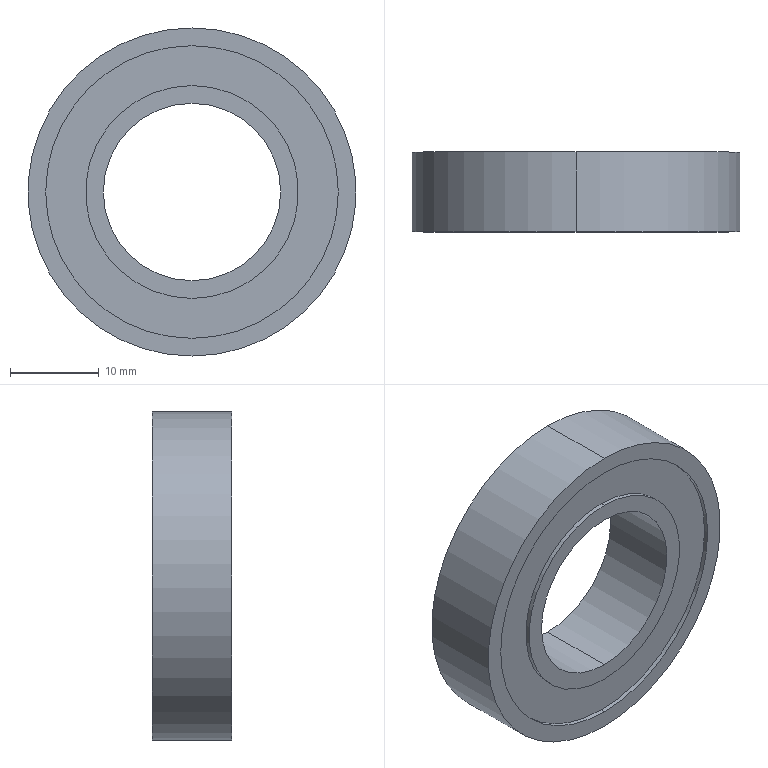Part | STEP file | Bearing 6904 | 1 solid | 18 faces | box 37 x 9 x 37 mm | volume 6447 mm3 | cylinder 12 | plane 6 | commonest cylinder face diameters 24 x4 33 x4 20 x2 37 x2
STEP:
#1=CARTESIAN_POINT('',(0.,0.,0.));
#2=DIRECTION('',(0.,0.,1.));
#3=DIRECTION('',(1.,0.,0.));
#4=AXIS2_PLACEMENT_3D('',#1,#2,#3);
#5=CARTESIAN_POINT('',(0.,-4.,12.));
#6=VERTEX_POINT('',#5);
#7=CARTESIAN_POINT('',(0.,-4.,-12.));
#8=VERTEX_POINT('',#7);
#9=CARTESIAN_POINT('',(0.,-4.,0.));
#10=DIRECTION('',(0.,1.,0.));
#11=DIRECTION('',(0.,0.,1.));
#12=AXIS2_PLACEMENT_3D('',#9,#10,#11);
#13=CIRCLE('',#12,12.);
#14=CARTESIAN_POINT('',(0.,-4.,0.));
#15=DIRECTION('',(0.,-1.,0.));
#16=DIRECTION('',(0.,0.,-1.));
#17=AXIS2_PLACEMENT_3D('',#14,#15,#16);
#18=CYLINDRICAL_SURFACE('',#17,12.);
#19=CARTESIAN_POINT('',(3.142,0.));
#20=DIRECTION('',(-1.,0.));
#21=VECTOR('',#20,1.);
#22=LINE('',#19,#21);
#23=(GEOMETRIC_REPRESENTATION_CONTEXT(2)PARAMETRIC_REPRESENTATION_CONTEXT()REPRESENTATION_CONTEXT('',''));
#24=DEFINITIONAL_REPRESENTATION('',(#22),#23);
#25=PCURVE('',#18,#24);
#26=CARTESIAN_POINT('',(0.,-4.,0.));
#27=DIRECTION('',(0.,-1.,0.));
#28=DIRECTION('',(0.,0.,1.));
#29=AXIS2_PLACEMENT_3D('',#26,#27,#28);
#30=PLANE('',#29);
#31=CARTESIAN_POINT('',(12.,0.));
#32=CARTESIAN_POINT('',(12.,-20.785));
#33=CARTESIAN_POINT('',(-6.,-10.392));
#34=CARTESIAN_POINT('',(-24.,0.));
#35=CARTESIAN_POINT('',(-6.,10.392));
#36=CARTESIAN_POINT('',(12.,20.785));
#37=CARTESIAN_POINT('',(12.,0.));
#38=(BOUNDED_CURVE()B_SPLINE_CURVE(2,(#31,#32,#33,#34,#35,#36,#37),.UNSPECIFIED.,.T.,.F.)B_SPLINE_CURVE_WITH_KNOTS((1,2,2,2,2,1),(-2.094,0.,2.094,4.189,6.283,8.378),.UNSPECIFIED.)CURVE()GEOMETRIC_REPRESENTATION_ITEM()RATIONAL_B_SPLINE_CURVE((1.,0.5,1.,0.5,1.,0.5,1.))REPRESENTATION_ITEM(''));
#39=(GEOMETRIC_REPRESENTATION_CONTEXT(2)PARAMETRIC_REPRESENTATION_CONTEXT()REPRESENTATION_CONTEXT('',''));
#40=DEFINITIONAL_REPRESENTATION('',(#38),#39);
#41=PCURVE('',#30,#40);
#42=SURFACE_CURVE('',#13,(#25,#41),.PCURVE_S1.);
#43=EDGE_CURVE('',#6,#8,#42,.T.);
#44=ORIENTED_EDGE('',*,*,#43,.F.);
#45=CARTESIAN_POINT('',(0.,-4.5,12.));
#46=VERTEX_POINT('',#45);
#47=CARTESIAN_POINT('',(0.,-4.,12.));
#48=DIRECTION('',(0.,-1.,0.));
#49=VECTOR('',#48,1.);
#50=LINE('',#47,#49);
#51=CARTESIAN_POINT('',(3.142,0.));
#52=DIRECTION('',(0.,1.));
#53=VECTOR('',#52,1.);
#54=LINE('',#51,#53);
#55=(GEOMETRIC_REPRESENTATION_CONTEXT(2)PARAMETRIC_REPRESENTATION_CONTEXT()REPRESENTATION_CONTEXT('',''));
#56=DEFINITIONAL_REPRESENTATION('',(#54),#55);
#57=PCURVE('',#18,#56);
#58=CARTESIAN_POINT('',(0.,-4.,0.));
#59=DIRECTION('',(0.,-1.,0.));
#60=DIRECTION('',(0.,0.,-1.));
#61=AXIS2_PLACEMENT_3D('',#58,#59,#60);
#62=CYLINDRICAL_SURFACE('',#61,12.);
#63=CARTESIAN_POINT('',(3.142,0.));
#64=DIRECTION('',(0.,1.));
#65=VECTOR('',#64,1.);
#66=LINE('',#63,#65);
#67=(GEOMETRIC_REPRESENTATION_CONTEXT(2)PARAMETRIC_REPRESENTATION_CONTEXT()REPRESENTATION_CONTEXT('',''));
#68=DEFINITIONAL_REPRESENTATION('',(#66),#67);
#69=PCURVE('',#62,#68);
#70=SURFACE_CURVE('',#50,(#57,#69),.PCURVE_S1.);
#71=EDGE_CURVE('',#6,#46,#70,.T.);
#72=ORIENTED_EDGE('',*,*,#71,.T.);
#73=CARTESIAN_POINT('',(0.,-4.5,-12.));
#74=VERTEX_POINT('',#73);
#75=CARTESIAN_POINT('',(0.,-4.5,0.));
#76=DIRECTION('',(0.,1.,0.));
#77=DIRECTION('',(0.,0.,1.));
#78=AXIS2_PLACEMENT_3D('',#75,#76,#77);
#79=CIRCLE('',#78,12.);
#80=CARTESIAN_POINT('',(3.142,0.5));
#81=DIRECTION('',(-1.,0.));
#82=VECTOR('',#81,1.);
#83=LINE('',#80,#82);
#84=(GEOMETRIC_REPRESENTATION_CONTEXT(2)PARAMETRIC_REPRESENTATION_CONTEXT()REPRESENTATION_CONTEXT('',''));
#85=DEFINITIONAL_REPRESENTATION('',(#83),#84);
#86=PCURVE('',#18,#85);
#87=CARTESIAN_POINT('',(0.,-4.5,0.));
#88=DIRECTION('',(0.,1.,0.));
#89=DIRECTION('',(0.,0.,1.));
#90=AXIS2_PLACEMENT_3D('',#87,#88,#89);
#91=PLANE('',#90);
#92=CARTESIAN_POINT('',(0.,0.));
#93=DIRECTION('',(1.,0.));
#94=AXIS2_PLACEMENT_2D('',#92,#93);
#95=CIRCLE('',#94,12.);
#96=(GEOMETRIC_REPRESENTATION_CONTEXT(2)PARAMETRIC_REPRESENTATION_CONTEXT()REPRESENTATION_CONTEXT('',''));
#97=DEFINITIONAL_REPRESENTATION('',(#95),#96);
#98=PCURVE('',#91,#97);
#99=SURFACE_CURVE('',#79,(#86,#98),.PCURVE_S1.);
#100=EDGE_CURVE('',#46,#74,#99,.T.);
#101=ORIENTED_EDGE('',*,*,#100,.T.);
#102=CARTESIAN_POINT('',(0.,-4.,-12.));
#103=DIRECTION('',(0.,-1.,0.));
#104=VECTOR('',#103,1.);
#105=LINE('',#102,#104);
#106=CARTESIAN_POINT('',(0.,0.));
#107=DIRECTION('',(0.,1.));
#108=VECTOR('',#107,1.);
#109=LINE('',#106,#108);
#110=(GEOMETRIC_REPRESENTATION_CONTEXT(2)PARAMETRIC_REPRESENTATION_CONTEXT()REPRESENTATION_CONTEXT('',''));
#111=DEFINITIONAL_REPRESENTATION('',(#109),#110);
#112=PCURVE('',#18,#111);
#113=CARTESIAN_POINT('',(6.283,0.));
#114=DIRECTION('',(0.,1.));
#115=VECTOR('',#114,1.);
#116=LINE('',#113,#115);
#117=(GEOMETRIC_REPRESENTATION_CONTEXT(2)PARAMETRIC_REPRESENTATION_CONTEXT()REPRESENTATION_CONTEXT('',''));
#118=DEFINITIONAL_REPRESENTATION('',(#116),#117);
#119=PCURVE('',#62,#118);
#120=SURFACE_CURVE('',#105,(#112,#119),.PCURVE_S1.);
#121=EDGE_CURVE('',#8,#74,#120,.T.);
#122=ORIENTED_EDGE('',*,*,#121,.F.);
#123=EDGE_LOOP('',(#44,#72,#101,#122));
#124=FACE_BOUND('',#123,.T.);
#125=ADVANCED_FACE('',(#124),#18,.T.);
#126=CARTESIAN_POINT('',(0.,-4.,-16.5));
#127=VERTEX_POINT('',#126);
#128=CARTESIAN_POINT('',(0.,-4.5,-16.5));
#129=VERTEX_POINT('',#128);
#130=CARTESIAN_POINT('',(0.,-4.,-16.5));
#131=DIRECTION('',(0.,-1.,0.));
#132=VECTOR('',#131,1.);
#133=LINE('',#130,#132);
#134=CARTESIAN_POINT('',(0.,-4.,0.));
#135=DIRECTION('',(0.,-1.,0.));
#136=DIRECTION('',(0.,0.,-1.));
#137=AXIS2_PLACEMENT_3D('',#134,#135,#136);
#138=CYLINDRICAL_SURFACE('',#137,16.5);
#139=CARTESIAN_POINT('',(6.283,0.));
#140=DIRECTION('',(0.,1.));
#141=VECTOR('',#140,1.);
#142=LINE('',#139,#141);
#143=(GEOMETRIC_REPRESENTATION_CONTEXT(2)PARAMETRIC_REPRESENTATION_CONTEXT()REPRESENTATION_CONTEXT('',''));
#144=DEFINITIONAL_REPRESENTATION('',(#142),#143);
#145=PCURVE('',#138,#144);
#146=CARTESIAN_POINT('',(0.,-4.,0.));
#147=DIRECTION('',(0.,-1.,0.));
#148=DIRECTION('',(0.,0.,-1.));
#149=AXIS2_PLACEMENT_3D('',#146,#147,#148);
#150=CYLINDRICAL_SURFACE('',#149,16.5);
#151=CARTESIAN_POINT('',(0.,0.));
#152=DIRECTION('',(0.,1.));
#153=VECTOR('',#152,1.);
#154=LINE('',#151,#153);
#155=(GEOMETRIC_REPRESENTATION_CONTEXT(2)PARAMETRIC_REPRESENTATION_CONTEXT()REPRESENTATION_CONTEXT('',''));
#156=DEFINITIONAL_REPRESENTATION('',(#154),#155);
#157=PCURVE('',#150,#156);
#158=SURFACE_CURVE('',#133,(#145,#157),.PCURVE_S1.);
#159=EDGE_CURVE('',#127,#129,#158,.T.);
#160=ORIENTED_EDGE('',*,*,#159,.T.);
#161=CARTESIAN_POINT('',(0.,-4.5,16.5));
#162=VERTEX_POINT('',#161);
#163=CARTESIAN_POINT('',(0.,-4.5,0.));
#164=DIRECTION('',(0.,1.,0.));
#165=DIRECTION('',(0.,0.,1.));
#166=AXIS2_PLACEMENT_3D('',#163,#164,#165);
#167=CIRCLE('',#166,16.5);
#168=CARTESIAN_POINT('',(9.425,0.5));
#169=DIRECTION('',(-1.,0.));
#170=VECTOR('',#169,1.);
#171=LINE('',#168,#170);
#172=(GEOMETRIC_REPRESENTATION_CONTEXT(2)PARAMETRIC_REPRESENTATION_CONTEXT()REPRESENTATION_CONTEXT('',''));
#173=DEFINITIONAL_REPRESENTATION('',(#171),#172);
#174=PCURVE('',#138,#173);
#175=CARTESIAN_POINT('',(0.,-4.5,0.));
#176=DIRECTION('',(0.,1.,0.));
#177=DIRECTION('',(0.,0.,1.));
#178=AXIS2_PLACEMENT_3D('',#175,#176,#177);
#179=PLANE('',#178);
#180=CARTESIAN_POINT('',(0.,0.));
#181=DIRECTION('',(1.,0.));
#182=AXIS2_PLACEMENT_2D('',#180,#181);
#183=CIRCLE('',#182,16.5);
#184=(GEOMETRIC_REPRESENTATION_CONTEXT(2)PARAMETRIC_REPRESENTATION_CONTEXT()REPRESENTATION_CONTEXT('',''));
#185=DEFINITIONAL_REPRESENTATION('',(#183),#184);
#186=PCURVE('',#179,#185);
#187=SURFACE_CURVE('',#167,(#174,#186),.PCURVE_S1.);
#188=EDGE_CURVE('',#129,#162,#187,.T.);
#189=ORIENTED_EDGE('',*,*,#188,.T.);
#190=CARTESIAN_POINT('',(0.,-4.,16.5));
#191=VERTEX_POINT('',#190);
#192=CARTESIAN_POINT('',(0.,-4.,16.5));
#193=DIRECTION('',(0.,-1.,0.));
#194=VECTOR('',#193,1.);
#195=LINE('',#192,#194);
#196=CARTESIAN_POINT('',(3.142,0.));
#197=DIRECTION('',(0.,1.));
#198=VECTOR('',#197,1.);
#199=LINE('',#196,#198);
#200=(GEOMETRIC_REPRESENTATION_CONTEXT(2)PARAMETRIC_REPRESENTATION_CONTEXT()REPRESENTATION_CONTEXT('',''));
#201=DEFINITIONAL_REPRESENTATION('',(#199),#200);
#202=PCURVE('',#138,#201);
#203=CARTESIAN_POINT('',(3.142,0.));
#204=DIRECTION('',(0.,1.));
#205=VECTOR('',#204,1.);
#206=LINE('',#203,#205);
#207=(GEOMETRIC_REPRESENTATION_CONTEXT(2)PARAMETRIC_REPRESENTATION_CONTEXT()REPRESENTATION_CONTEXT('',''));
#208=DEFINITIONAL_REPRESENTATION('',(#206),#207);
#209=PCURVE('',#150,#208);
#210=SURFACE_CURVE('',#195,(#202,#209),.PCURVE_S1.);
#211=EDGE_CURVE('',#191,#162,#210,.T.);
#212=ORIENTED_EDGE('',*,*,#211,.F.);
#213=CARTESIAN_POINT('',(0.,-4.,0.));
#214=DIRECTION('',(0.,1.,0.));
#215=DIRECTION('',(0.,0.,1.));
#216=AXIS2_PLACEMENT_3D('',#213,#214,#215);
#217=CIRCLE('',#216,16.5);
#218=CARTESIAN_POINT('',(9.425,0.));
#219=DIRECTION('',(-1.,0.));
#220=VECTOR('',#219,1.);
#221=LINE('',#218,#220);
#222=(GEOMETRIC_REPRESENTATION_CONTEXT(2)PARAMETRIC_REPRESENTATION_CONTEXT()REPRESENTATION_CONTEXT('',''));
#223=DEFINITIONAL_REPRESENTATION('',(#221),#222);
#224=PCURVE('',#138,#223);
#225=CARTESIAN_POINT('',(16.5,0.));
#226=CARTESIAN_POINT('',(16.5,-28.579));
#227=CARTESIAN_POINT('',(-8.25,-14.289));
#228=CARTESIAN_POINT('',(-33.,0.));
#229=CARTESIAN_POINT('',(-8.25,14.289));
#230=CARTESIAN_POINT('',(16.5,28.579));
#231=CARTESIAN_POINT('',(16.5,0.));
#232=(BOUNDED_CURVE()B_SPLINE_CURVE(2,(#225,#226,#227,#228,#229,#230,#231),.UNSPECIFIED.,.T.,.F.)B_SPLINE_CURVE_WITH_KNOTS((1,2,2,2,2,1),(-2.094,0.,2.094,4.189,6.283,8.378),.UNSPECIFIED.)CURVE()GEOMETRIC_REPRESENTATION_ITEM()RATIONAL_B_SPLINE_CURVE((1.,0.5,1.,0.5,1.,0.5,1.))REPRESENTATION_ITEM(''));
#233=(GEOMETRIC_REPRESENTATION_CONTEXT(2)PARAMETRIC_REPRESENTATION_CONTEXT()REPRESENTATION_CONTEXT('',''));
#234=DEFINITIONAL_REPRESENTATION('',(#232),#233);
#235=PCURVE('',#30,#234);
#236=SURFACE_CURVE('',#217,(#224,#235),.PCURVE_S1.);
#237=EDGE_CURVE('',#127,#191,#236,.T.);
#238=ORIENTED_EDGE('',*,*,#237,.F.);
#239=EDGE_LOOP('',(#160,#189,#212,#238));
#240=FACE_BOUND('',#239,.F.);
#241=ADVANCED_FACE('',(#240),#138,.F.);
#242=CARTESIAN_POINT('',(0.,4.,12.));
#243=VERTEX_POINT('',#242);
#244=CARTESIAN_POINT('',(0.,4.,-12.));
#245=VERTEX_POINT('',#244);
#246=CARTESIAN_POINT('',(0.,4.,0.));
#247=DIRECTION('',(0.,1.,0.));
#248=DIRECTION('',(0.,0.,1.));
#249=AXIS2_PLACEMENT_3D('',#246,#247,#248);
#250=CIRCLE('',#249,12.);
#251=CARTESIAN_POINT('',(0.,4.,0.));
#252=DIRECTION('',(0.,1.,0.));
#253=DIRECTION('',(0.,0.,1.));
#254=AXIS2_PLACEMENT_3D('',#251,#252,#253);
#255=CYLINDRICAL_SURFACE('',#254,12.);
#256=CARTESIAN_POINT('',(0.,0.));
#257=DIRECTION('',(1.,0.));
#258=VECTOR('',#257,1.);
#259=LINE('',#256,#258);
#260=(GEOMETRIC_REPRESENTATION_CONTEXT(2)PARAMETRIC_REPRESENTATION_CONTEXT()REPRESENTATION_CONTEXT('',''));
#261=DEFINITIONAL_REPRESENTATION('',(#259),#260);
#262=PCURVE('',#255,#261);
#263=CARTESIAN_POINT('',(0.,4.,0.));
#264=DIRECTION('',(0.,1.,0.));
#265=DIRECTION('',(0.,0.,1.));
#266=AXIS2_PLACEMENT_3D('',#263,#264,#265);
#267=PLANE('',#266);
#268=CARTESIAN_POINT('',(0.,0.));
#269=DIRECTION('',(1.,0.));
#270=AXIS2_PLACEMENT_2D('',#268,#269);
#271=CIRCLE('',#270,12.);
#272=(GEOMETRIC_REPRESENTATION_CONTEXT(2)PARAMETRIC_REPRESENTATION_CONTEXT()REPRESENTATION_CONTEXT('',''));
#273=DEFINITIONAL_REPRESENTATION('',(#271),#272);
#274=PCURVE('',#267,#273);
#275=SURFACE_CURVE('',#250,(#262,#274),.PCURVE_S1.);
#276=EDGE_CURVE('',#243,#245,#275,.T.);
#277=ORIENTED_EDGE('',*,*,#276,.T.);
#278=CARTESIAN_POINT('',(0.,4.5,-12.));
#279=VERTEX_POINT('',#278);
#280=CARTESIAN_POINT('',(0.,4.,-12.));
#281=DIRECTION('',(0.,1.,0.));
#282=VECTOR('',#281,1.);
#283=LINE('',#280,#282);
#284=CARTESIAN_POINT('',(3.142,0.));
#285=DIRECTION('',(0.,1.));
#286=VECTOR('',#285,1.);
#287=LINE('',#284,#286);
#288=(GEOMETRIC_REPRESENTATION_CONTEXT(2)PARAMETRIC_REPRESENTATION_CONTEXT()REPRESENTATION_CONTEXT('',''));
#289=DEFINITIONAL_REPRESENTATION('',(#287),#288);
#290=PCURVE('',#255,#289);
#291=CARTESIAN_POINT('',(0.,4.,0.));
#292=DIRECTION('',(0.,1.,0.));
#293=DIRECTION('',(0.,0.,1.));
#294=AXIS2_PLACEMENT_3D('',#291,#292,#293);
#295=CYLINDRICAL_SURFACE('',#294,12.);
#296=CARTESIAN_POINT('',(3.142,0.));
#297=DIRECTION('',(0.,1.));
#298=VECTOR('',#297,1.);
#299=LINE('',#296,#298);
#300=(GEOMETRIC_REPRESENTATION_CONTEXT(2)PARAMETRIC_REPRESENTATION_CONTEXT()REPRESENTATION_CONTEXT('',''));
#301=DEFINITIONAL_REPRESENTATION('',(#299),#300);
#302=PCURVE('',#295,#301);
#303=SURFACE_CURVE('',#283,(#290,#302),.PCURVE_S1.);
#304=EDGE_CURVE('',#245,#279,#303,.T.);
#305=ORIENTED_EDGE('',*,*,#304,.T.);
#306=CARTESIAN_POINT('',(0.,4.5,12.));
#307=VERTEX_POINT('',#306);
#308=CARTESIAN_POINT('',(0.,4.5,0.));
#309=DIRECTION('',(0.,1.,0.));
#310=DIRECTION('',(0.,0.,1.));
#311=AXIS2_PLACEMENT_3D('',#308,#309,#310);
#312=CIRCLE('',#311,12.);
#313=CARTESIAN_POINT('',(0.,0.5));
#314=DIRECTION('',(1.,0.));
#315=VECTOR('',#314,1.);
#316=LINE('',#313,#315);
#317=(GEOMETRIC_REPRESENTATION_CONTEXT(2)PARAMETRIC_REPRESENTATION_CONTEXT()REPRESENTATION_CONTEXT('',''));
#318=DEFINITIONAL_REPRESENTATION('',(#316),#317);
#319=PCURVE('',#255,#318);
#320=CARTESIAN_POINT('',(0.,4.5,0.));
#321=DIRECTION('',(0.,1.,0.));
#322=DIRECTION('',(0.,0.,1.));
#323=AXIS2_PLACEMENT_3D('',#320,#321,#322);
#324=PLANE('',#323);
#325=CARTESIAN_POINT('',(0.,0.));
#326=DIRECTION('',(1.,0.));
#327=AXIS2_PLACEMENT_2D('',#325,#326);
#328=CIRCLE('',#327,12.);
#329=(GEOMETRIC_REPRESENTATION_CONTEXT(2)PARAMETRIC_REPRESENTATION_CONTEXT()REPRESENTATION_CONTEXT('',''));
#330=DEFINITIONAL_REPRESENTATION('',(#328),#329);
#331=PCURVE('',#324,#330);
#332=SURFACE_CURVE('',#312,(#319,#331),.PCURVE_S1.);
#333=EDGE_CURVE('',#307,#279,#332,.T.);
#334=ORIENTED_EDGE('',*,*,#333,.F.);
#335=CARTESIAN_POINT('',(0.,4.,12.));
#336=DIRECTION('',(0.,1.,0.));
#337=VECTOR('',#336,1.);
#338=LINE('',#335,#337);
#339=CARTESIAN_POINT('',(0.,0.));
#340=DIRECTION('',(0.,1.));
#341=VECTOR('',#340,1.);
#342=LINE('',#339,#341);
#343=(GEOMETRIC_REPRESENTATION_CONTEXT(2)PARAMETRIC_REPRESENTATION_CONTEXT()REPRESENTATION_CONTEXT('',''));
#344=DEFINITIONAL_REPRESENTATION('',(#342),#343);
#345=PCURVE('',#255,#344);
#346=CARTESIAN_POINT('',(6.283,0.));
#347=DIRECTION('',(0.,1.));
#348=VECTOR('',#347,1.);
#349=LINE('',#346,#348);
#350=(GEOMETRIC_REPRESENTATION_CONTEXT(2)PARAMETRIC_REPRESENTATION_CONTEXT()REPRESENTATION_CONTEXT('',''));
#351=DEFINITIONAL_REPRESENTATION('',(#349),#350);
#352=PCURVE('',#295,#351);
#353=SURFACE_CURVE('',#338,(#345,#352),.PCURVE_S1.);
#354=EDGE_CURVE('',#243,#307,#353,.T.);
#355=ORIENTED_EDGE('',*,*,#354,.F.);
#356=EDGE_LOOP('',(#277,#305,#334,#355));
#357=FACE_BOUND('',#356,.T.);
#358=ADVANCED_FACE('',(#357),#255,.T.);
#359=CARTESIAN_POINT('',(0.,4.,16.5));
#360=VERTEX_POINT('',#359);
#361=CARTESIAN_POINT('',(0.,4.5,16.5));
#362=VERTEX_POINT('',#361);
#363=CARTESIAN_POINT('',(0.,4.,16.5));
#364=DIRECTION('',(0.,1.,0.));
#365=VECTOR('',#364,1.);
#366=LINE('',#363,#365);
#367=CARTESIAN_POINT('',(0.,4.,0.));
#368=DIRECTION('',(0.,1.,0.));
#369=DIRECTION('',(0.,0.,1.));
#370=AXIS2_PLACEMENT_3D('',#367,#368,#369);
#371=CYLINDRICAL_SURFACE('',#370,16.5);
#372=CARTESIAN_POINT('',(6.283,0.));
#373=DIRECTION('',(0.,1.));
#374=VECTOR('',#373,1.);
#375=LINE('',#372,#374);
#376=(GEOMETRIC_REPRESENTATION_CONTEXT(2)PARAMETRIC_REPRESENTATION_CONTEXT()REPRESENTATION_CONTEXT('',''));
#377=DEFINITIONAL_REPRESENTATION('',(#375),#376);
#378=PCURVE('',#371,#377);
#379=CARTESIAN_POINT('',(0.,4.,0.));
#380=DIRECTION('',(0.,1.,0.));
#381=DIRECTION('',(0.,0.,1.));
#382=AXIS2_PLACEMENT_3D('',#379,#380,#381);
#383=CYLINDRICAL_SURFACE('',#382,16.5);
#384=CARTESIAN_POINT('',(0.,0.));
#385=DIRECTION('',(0.,1.));
#386=VECTOR('',#385,1.);
#387=LINE('',#384,#386);
#388=(GEOMETRIC_REPRESENTATION_CONTEXT(2)PARAMETRIC_REPRESENTATION_CONTEXT()REPRESENTATION_CONTEXT('',''));
#389=DEFINITIONAL_REPRESENTATION('',(#387),#388);
#390=PCURVE('',#383,#389);
#391=SURFACE_CURVE('',#366,(#378,#390),.PCURVE_S1.);
#392=EDGE_CURVE('',#360,#362,#391,.T.);
#393=ORIENTED_EDGE('',*,*,#392,.T.);
#394=CARTESIAN_POINT('',(0.,4.5,-16.5));
#395=VERTEX_POINT('',#394);
#396=CARTESIAN_POINT('',(0.,4.5,0.));
#397=DIRECTION('',(0.,1.,0.));
#398=DIRECTION('',(0.,0.,1.));
#399=AXIS2_PLACEMENT_3D('',#396,#397,#398);
#400=CIRCLE('',#399,16.5);
#401=CARTESIAN_POINT('',(0.,0.5));
#402=DIRECTION('',(1.,0.));
#403=VECTOR('',#402,1.);
#404=LINE('',#401,#403);
#405=(GEOMETRIC_REPRESENTATION_CONTEXT(2)PARAMETRIC_REPRESENTATION_CONTEXT()REPRESENTATION_CONTEXT('',''));
#406=DEFINITIONAL_REPRESENTATION('',(#404),#405);
#407=PCURVE('',#371,#406);
#408=CARTESIAN_POINT('',(0.,4.5,0.));
#409=DIRECTION('',(0.,1.,0.));
#410=DIRECTION('',(0.,0.,1.));
#411=AXIS2_PLACEMENT_3D('',#408,#409,#410);
#412=PLANE('',#411);
#413=CARTESIAN_POINT('',(0.,0.));
#414=DIRECTION('',(1.,0.));
#415=AXIS2_PLACEMENT_2D('',#413,#414);
#416=CIRCLE('',#415,16.5);
#417=(GEOMETRIC_REPRESENTATION_CONTEXT(2)PARAMETRIC_REPRESENTATION_CONTEXT()REPRESENTATION_CONTEXT('',''));
#418=DEFINITIONAL_REPRESENTATION('',(#416),#417);
#419=PCURVE('',#412,#418);
#420=SURFACE_CURVE('',#400,(#407,#419),.PCURVE_S1.);
#421=EDGE_CURVE('',#395,#362,#420,.T.);
#422=ORIENTED_EDGE('',*,*,#421,.F.);
#423=CARTESIAN_POINT('',(0.,4.,-16.5));
#424=VERTEX_POINT('',#423);
#425=CARTESIAN_POINT('',(0.,4.,-16.5));
#426=DIRECTION('',(0.,1.,0.));
#427=VECTOR('',#426,1.);
#428=LINE('',#425,#427);
#429=CARTESIAN_POINT('',(3.142,0.));
#430=DIRECTION('',(0.,1.));
#431=VECTOR('',#430,1.);
#432=LINE('',#429,#431);
#433=(GEOMETRIC_REPRESENTATION_CONTEXT(2)PARAMETRIC_REPRESENTATION_CONTEXT()REPRESENTATION_CONTEXT('',''));
#434=DEFINITIONAL_REPRESENTATION('',(#432),#433);
#435=PCURVE('',#371,#434);
#436=CARTESIAN_POINT('',(3.142,0.));
#437=DIRECTION('',(0.,1.));
#438=VECTOR('',#437,1.);
#439=LINE('',#436,#438);
#440=(GEOMETRIC_REPRESENTATION_CONTEXT(2)PARAMETRIC_REPRESENTATION_CONTEXT()REPRESENTATION_CONTEXT('',''));
#441=DEFINITIONAL_REPRESENTATION('',(#439),#440);
#442=PCURVE('',#383,#441);
#443=SURFACE_CURVE('',#428,(#435,#442),.PCURVE_S1.);
#444=EDGE_CURVE('',#424,#395,#443,.T.);
#445=ORIENTED_EDGE('',*,*,#444,.F.);
#446=CARTESIAN_POINT('',(0.,4.,0.));
#447=DIRECTION('',(0.,1.,0.));
#448=DIRECTION('',(0.,0.,1.));
#449=AXIS2_PLACEMENT_3D('',#446,#447,#448);
#450=CIRCLE('',#449,16.5);
#451=CARTESIAN_POINT('',(0.,0.));
#452=DIRECTION('',(1.,0.));
#453=VECTOR('',#452,1.);
#454=LINE('',#451,#453);
#455=(GEOMETRIC_REPRESENTATION_CONTEXT(2)PARAMETRIC_REPRESENTATION_CONTEXT()REPRESENTATION_CONTEXT('',''));
#456=DEFINITIONAL_REPRESENTATION('',(#454),#455);
#457=PCURVE('',#371,#456);
#458=CARTESIAN_POINT('',(0.,0.));
#459=DIRECTION('',(1.,0.));
#460=AXIS2_PLACEMENT_2D('',#458,#459);
#461=CIRCLE('',#460,16.5);
#462=(GEOMETRIC_REPRESENTATION_CONTEXT(2)PARAMETRIC_REPRESENTATION_CONTEXT()REPRESENTATION_CONTEXT('',''));
#463=DEFINITIONAL_REPRESENTATION('',(#461),#462);
#464=PCURVE('',#267,#463);
#465=SURFACE_CURVE('',#450,(#457,#464),.PCURVE_S1.);
#466=EDGE_CURVE('',#424,#360,#465,.T.);
#467=ORIENTED_EDGE('',*,*,#466,.T.);
#468=EDGE_LOOP('',(#393,#422,#445,#467));
#469=FACE_BOUND('',#468,.F.);
#470=ADVANCED_FACE('',(#469),#371,.F.);
#471=CARTESIAN_POINT('',(0.,4.5,-10.));
#472=VERTEX_POINT('',#471);
#473=CARTESIAN_POINT('',(0.,-4.5,-10.));
#474=VERTEX_POINT('',#473);
#475=CARTESIAN_POINT('',(0.,4.5,-10.));
#476=DIRECTION('',(0.,-1.,0.));
#477=VECTOR('',#476,1.);
#478=LINE('',#475,#477);
#479=CARTESIAN_POINT('',(0.,4.5,0.));
#480=DIRECTION('',(0.,-1.,0.));
#481=DIRECTION('',(0.,0.,-1.));
#482=AXIS2_PLACEMENT_3D('',#479,#480,#481);
#483=CYLINDRICAL_SURFACE('',#482,10.);
#484=CARTESIAN_POINT('',(6.283,0.));
#485=DIRECTION('',(0.,1.));
#486=VECTOR('',#485,1.);
#487=LINE('',#484,#486);
#488=(GEOMETRIC_REPRESENTATION_CONTEXT(2)PARAMETRIC_REPRESENTATION_CONTEXT()REPRESENTATION_CONTEXT('',''));
#489=DEFINITIONAL_REPRESENTATION('',(#487),#488);
#490=PCURVE('',#483,#489);
#491=CARTESIAN_POINT('',(0.,4.5,0.));
#492=DIRECTION('',(0.,-1.,0.));
#493=DIRECTION('',(0.,0.,-1.));
#494=AXIS2_PLACEMENT_3D('',#491,#492,#493);
#495=CYLINDRICAL_SURFACE('',#494,10.);
#496=CARTESIAN_POINT('',(0.,0.));
#497=DIRECTION('',(0.,1.));
#498=VECTOR('',#497,1.);
#499=LINE('',#496,#498);
#500=(GEOMETRIC_REPRESENTATION_CONTEXT(2)PARAMETRIC_REPRESENTATION_CONTEXT()REPRESENTATION_CONTEXT('',''));
#501=DEFINITIONAL_REPRESENTATION('',(#499),#500);
#502=PCURVE('',#495,#501);
#503=SURFACE_CURVE('',#478,(#490,#502),.PCURVE_S1.);
#504=EDGE_CURVE('',#472,#474,#503,.T.);
#505=ORIENTED_EDGE('',*,*,#504,.T.);
#506=CARTESIAN_POINT('',(0.,-4.5,10.));
#507=VERTEX_POINT('',#506);
#508=CARTESIAN_POINT('',(0.,-4.5,0.));
#509=DIRECTION('',(0.,1.,0.));
#510=DIRECTION('',(0.,0.,1.));
#511=AXIS2_PLACEMENT_3D('',#508,#509,#510);
#512=CIRCLE('',#511,10.);
#513=CARTESIAN_POINT('',(9.425,9.));
#514=DIRECTION('',(-1.,0.));
#515=VECTOR('',#514,1.);
#516=LINE('',#513,#515);
#517=(GEOMETRIC_REPRESENTATION_CONTEXT(2)PARAMETRIC_REPRESENTATION_CONTEXT()REPRESENTATION_CONTEXT('',''));
#518=DEFINITIONAL_REPRESENTATION('',(#516),#517);
#519=PCURVE('',#483,#518);
#520=CARTESIAN_POINT('',(0.,0.));
#521=DIRECTION('',(1.,0.));
#522=AXIS2_PLACEMENT_2D('',#520,#521);
#523=CIRCLE('',#522,10.);
#524=(GEOMETRIC_REPRESENTATION_CONTEXT(2)PARAMETRIC_REPRESENTATION_CONTEXT()REPRESENTATION_CONTEXT('',''));
#525=DEFINITIONAL_REPRESENTATION('',(#523),#524);
#526=PCURVE('',#91,#525);
#527=SURFACE_CURVE('',#512,(#519,#526),.PCURVE_S1.);
#528=EDGE_CURVE('',#474,#507,#527,.T.);
#529=ORIENTED_EDGE('',*,*,#528,.T.);
#530=CARTESIAN_POINT('',(0.,4.5,10.));
#531=VERTEX_POINT('',#530);
#532=CARTESIAN_POINT('',(0.,4.5,10.));
#533=DIRECTION('',(0.,-1.,0.));
#534=VECTOR('',#533,1.);
#535=LINE('',#532,#534);
#536=CARTESIAN_POINT('',(3.142,0.));
#537=DIRECTION('',(0.,1.));
#538=VECTOR('',#537,1.);
#539=LINE('',#536,#538);
#540=(GEOMETRIC_REPRESENTATION_CONTEXT(2)PARAMETRIC_REPRESENTATION_CONTEXT()REPRESENTATION_CONTEXT('',''));
#541=DEFINITIONAL_REPRESENTATION('',(#539),#540);
#542=PCURVE('',#483,#541);
#543=CARTESIAN_POINT('',(3.142,0.));
#544=DIRECTION('',(0.,1.));
#545=VECTOR('',#544,1.);
#546=LINE('',#543,#545);
#547=(GEOMETRIC_REPRESENTATION_CONTEXT(2)PARAMETRIC_REPRESENTATION_CONTEXT()REPRESENTATION_CONTEXT('',''));
#548=DEFINITIONAL_REPRESENTATION('',(#546),#547);
#549=PCURVE('',#495,#548);
#550=SURFACE_CURVE('',#535,(#542,#549),.PCURVE_S1.);
#551=EDGE_CURVE('',#531,#507,#550,.T.);
#552=ORIENTED_EDGE('',*,*,#551,.F.);
#553=CARTESIAN_POINT('',(0.,4.5,0.));
#554=DIRECTION('',(0.,1.,0.));
#555=DIRECTION('',(0.,0.,1.));
#556=AXIS2_PLACEMENT_3D('',#553,#554,#555);
#557=CIRCLE('',#556,10.);
#558=CARTESIAN_POINT('',(9.425,0.));
#559=DIRECTION('',(-1.,0.));
#560=VECTOR('',#559,1.);
#561=LINE('',#558,#560);
#562=(GEOMETRIC_REPRESENTATION_CONTEXT(2)PARAMETRIC_REPRESENTATION_CONTEXT()REPRESENTATION_CONTEXT('',''));
#563=DEFINITIONAL_REPRESENTATION('',(#561),#562);
#564=PCURVE('',#483,#563);
#565=CARTESIAN_POINT('',(0.,0.));
#566=DIRECTION('',(1.,0.));
#567=AXIS2_PLACEMENT_2D('',#565,#566);
#568=CIRCLE('',#567,10.);
#569=(GEOMETRIC_REPRESENTATION_CONTEXT(2)PARAMETRIC_REPRESENTATION_CONTEXT()REPRESENTATION_CONTEXT('',''));
#570=DEFINITIONAL_REPRESENTATION('',(#568),#569);
#571=PCURVE('',#324,#570);
#572=SURFACE_CURVE('',#557,(#564,#571),.PCURVE_S1.);
#573=EDGE_CURVE('',#472,#531,#572,.T.);
#574=ORIENTED_EDGE('',*,*,#573,.F.);
#575=EDGE_LOOP('',(#505,#529,#552,#574));
#576=FACE_BOUND('',#575,.F.);
#577=ADVANCED_FACE('',(#576),#483,.F.);
#578=CARTESIAN_POINT('',(0.,4.5,18.5));
#579=VERTEX_POINT('',#578);
#580=CARTESIAN_POINT('',(0.,4.5,-18.5));
#581=VERTEX_POINT('',#580);
#582=CARTESIAN_POINT('',(0.,4.5,0.));
#583=DIRECTION('',(0.,1.,0.));
#584=DIRECTION('',(0.,0.,1.));
#585=AXIS2_PLACEMENT_3D('',#582,#583,#584);
#586=CIRCLE('',#585,18.5);
#587=CARTESIAN_POINT('',(0.,4.5,0.));
#588=DIRECTION('',(0.,-1.,0.));
#589=DIRECTION('',(0.,0.,-1.));
#590=AXIS2_PLACEMENT_3D('',#587,#588,#589);
#591=CYLINDRICAL_SURFACE('',#590,18.5);
#592=CARTESIAN_POINT('',(3.142,0.));
#593=DIRECTION('',(-1.,0.));
#594=VECTOR('',#593,1.);
#595=LINE('',#592,#594);
#596=(GEOMETRIC_REPRESENTATION_CONTEXT(2)PARAMETRIC_REPRESENTATION_CONTEXT()REPRESENTATION_CONTEXT('',''));
#597=DEFINITIONAL_REPRESENTATION('',(#595),#596);
#598=PCURVE('',#591,#597);
#599=CARTESIAN_POINT('',(0.,0.));
#600=DIRECTION('',(1.,0.));
#601=AXIS2_PLACEMENT_2D('',#599,#600);
#602=CIRCLE('',#601,18.5);
#603=(GEOMETRIC_REPRESENTATION_CONTEXT(2)PARAMETRIC_REPRESENTATION_CONTEXT()REPRESENTATION_CONTEXT('',''));
#604=DEFINITIONAL_REPRESENTATION('',(#602),#603);
#605=PCURVE('',#412,#604);
#606=SURFACE_CURVE('',#586,(#598,#605),.PCURVE_S1.);
#607=EDGE_CURVE('',#579,#581,#606,.T.);
#608=ORIENTED_EDGE('',*,*,#607,.F.);
#609=CARTESIAN_POINT('',(0.,-4.5,18.5));
#610=VERTEX_POINT('',#609);
#611=CARTESIAN_POINT('',(0.,4.5,18.5));
#612=DIRECTION('',(0.,-1.,0.));
#613=VECTOR('',#612,1.);
#614=LINE('',#611,#613);
#615=CARTESIAN_POINT('',(3.142,0.));
#616=DIRECTION('',(0.,1.));
#617=VECTOR('',#616,1.);
#618=LINE('',#615,#617);
#619=(GEOMETRIC_REPRESENTATION_CONTEXT(2)PARAMETRIC_REPRESENTATION_CONTEXT()REPRESENTATION_CONTEXT('',''));
#620=DEFINITIONAL_REPRESENTATION('',(#618),#619);
#621=PCURVE('',#591,#620);
#622=CARTESIAN_POINT('',(0.,4.5,0.));
#623=DIRECTION('',(0.,-1.,0.));
#624=DIRECTION('',(0.,0.,-1.));
#625=AXIS2_PLACEMENT_3D('',#622,#623,#624);
#626=CYLINDRICAL_SURFACE('',#625,18.5);
#627=CARTESIAN_POINT('',(3.142,0.));
#628=DIRECTION('',(0.,1.));
#629=VECTOR('',#628,1.);
#630=LINE('',#627,#629);
#631=(GEOMETRIC_REPRESENTATION_CONTEXT(2)PARAMETRIC_REPRESENTATION_CONTEXT()REPRESENTATION_CONTEXT('',''));
#632=DEFINITIONAL_REPRESENTATION('',(#630),#631);
#633=PCURVE('',#626,#632);
#634=SURFACE_CURVE('',#614,(#621,#633),.PCURVE_S1.);
#635=EDGE_CURVE('',#579,#610,#634,.T.);
#636=ORIENTED_EDGE('',*,*,#635,.T.);
#637=CARTESIAN_POINT('',(0.,-4.5,-18.5));
#638=VERTEX_POINT('',#637);
#639=CARTESIAN_POINT('',(0.,-4.5,0.));
#640=DIRECTION('',(0.,1.,0.));
#641=DIRECTION('',(0.,0.,1.));
#642=AXIS2_PLACEMENT_3D('',#639,#640,#641);
#643=CIRCLE('',#642,18.5);
#644=CARTESIAN_POINT('',(3.142,9.));
#645=DIRECTION('',(-1.,0.));
#646=VECTOR('',#645,1.);
#647=LINE('',#644,#646);
#648=(GEOMETRIC_REPRESENTATION_CONTEXT(2)PARAMETRIC_REPRESENTATION_CONTEXT()REPRESENTATION_CONTEXT('',''));
#649=DEFINITIONAL_REPRESENTATION('',(#647),#648);
#650=PCURVE('',#591,#649);
#651=CARTESIAN_POINT('',(0.,0.));
#652=DIRECTION('',(1.,0.));
#653=AXIS2_PLACEMENT_2D('',#651,#652);
#654=CIRCLE('',#653,18.5);
#655=(GEOMETRIC_REPRESENTATION_CONTEXT(2)PARAMETRIC_REPRESENTATION_CONTEXT()REPRESENTATION_CONTEXT('',''));
#656=DEFINITIONAL_REPRESENTATION('',(#654),#655);
#657=PCURVE('',#179,#656);
#658=SURFACE_CURVE('',#643,(#650,#657),.PCURVE_S1.);
#659=EDGE_CURVE('',#610,#638,#658,.T.);
#660=ORIENTED_EDGE('',*,*,#659,.T.);
#661=CARTESIAN_POINT('',(0.,4.5,-18.5));
#662=DIRECTION('',(0.,-1.,0.));
#663=VECTOR('',#662,1.);
#664=LINE('',#661,#663);
#665=CARTESIAN_POINT('',(0.,0.));
#666=DIRECTION('',(0.,1.));
#667=VECTOR('',#666,1.);
#668=LINE('',#665,#667);
#669=(GEOMETRIC_REPRESENTATION_CONTEXT(2)PARAMETRIC_REPRESENTATION_CONTEXT()REPRESENTATION_CONTEXT('',''));
#670=DEFINITIONAL_REPRESENTATION('',(#668),#669);
#671=PCURVE('',#591,#670);
#672=CARTESIAN_POINT('',(6.283,0.));
#673=DIRECTION('',(0.,1.));
#674=VECTOR('',#673,1.);
#675=LINE('',#672,#674);
#676=(GEOMETRIC_REPRESENTATION_CONTEXT(2)PARAMETRIC_REPRESENTATION_CONTEXT()REPRESENTATION_CONTEXT('',''));
#677=DEFINITIONAL_REPRESENTATION('',(#675),#676);
#678=PCURVE('',#626,#677);
#679=SURFACE_CURVE('',#664,(#671,#678),.PCURVE_S1.);
#680=EDGE_CURVE('',#581,#638,#679,.T.);
#681=ORIENTED_EDGE('',*,*,#680,.F.);
#682=EDGE_LOOP('',(#608,#636,#660,#681));
#683=FACE_BOUND('',#682,.T.);
#684=ADVANCED_FACE('',(#683),#591,.T.);
#685=ORIENTED_EDGE('',*,*,#528,.T.);
#686=CARTESIAN_POINT('',(0.,-4.5,0.));
#687=DIRECTION('',(0.,1.,0.));
#688=DIRECTION('',(0.,0.,1.));
#689=AXIS2_PLACEMENT_3D('',#686,#687,#688);
#690=CIRCLE('',#689,10.);
#691=CARTESIAN_POINT('',(0.,0.));
#692=DIRECTION('',(1.,0.));
#693=AXIS2_PLACEMENT_2D('',#691,#692);
#694=CIRCLE('',#693,10.);
#695=(GEOMETRIC_REPRESENTATION_CONTEXT(2)PARAMETRIC_REPRESENTATION_CONTEXT()REPRESENTATION_CONTEXT('',''));
#696=DEFINITIONAL_REPRESENTATION('',(#694),#695);
#697=PCURVE('',#91,#696);
#698=CARTESIAN_POINT('',(3.142,9.));
#699=DIRECTION('',(-1.,0.));
#700=VECTOR('',#699,1.);
#701=LINE('',#698,#700);
#702=(GEOMETRIC_REPRESENTATION_CONTEXT(2)PARAMETRIC_REPRESENTATION_CONTEXT()REPRESENTATION_CONTEXT('',''));
#703=DEFINITIONAL_REPRESENTATION('',(#701),#702);
#704=PCURVE('',#495,#703);
#705=SURFACE_CURVE('',#690,(#697,#704),.PCURVE_S1.);
#706=EDGE_CURVE('',#507,#474,#705,.T.);
#707=ORIENTED_EDGE('',*,*,#706,.T.);
#708=EDGE_LOOP('',(#685,#707));
#709=FACE_BOUND('',#708,.T.);
#710=CARTESIAN_POINT('',(0.,-4.5,0.));
#711=DIRECTION('',(0.,1.,0.));
#712=DIRECTION('',(0.,0.,1.));
#713=AXIS2_PLACEMENT_3D('',#710,#711,#712);
#714=CIRCLE('',#713,12.);
#715=CARTESIAN_POINT('',(0.,0.));
#716=DIRECTION('',(1.,0.));
#717=AXIS2_PLACEMENT_2D('',#715,#716);
#718=CIRCLE('',#717,12.);
#719=(GEOMETRIC_REPRESENTATION_CONTEXT(2)PARAMETRIC_REPRESENTATION_CONTEXT()REPRESENTATION_CONTEXT('',''));
#720=DEFINITIONAL_REPRESENTATION('',(#718),#719);
#721=PCURVE('',#91,#720);
#722=CARTESIAN_POINT('',(9.425,0.5));
#723=DIRECTION('',(-1.,0.));
#724=VECTOR('',#723,1.);
#725=LINE('',#722,#724);
#726=(GEOMETRIC_REPRESENTATION_CONTEXT(2)PARAMETRIC_REPRESENTATION_CONTEXT()REPRESENTATION_CONTEXT('',''));
#727=DEFINITIONAL_REPRESENTATION('',(#725),#726);
#728=PCURVE('',#62,#727);
#729=SURFACE_CURVE('',#714,(#721,#728),.PCURVE_S1.);
#730=EDGE_CURVE('',#74,#46,#729,.T.);
#731=ORIENTED_EDGE('',*,*,#730,.F.);
#732=ORIENTED_EDGE('',*,*,#100,.F.);
#733=EDGE_LOOP('',(#731,#732));
#734=FACE_BOUND('',#733,.T.);
#735=ADVANCED_FACE('',(#709,#734),#91,.F.);
#736=ORIENTED_EDGE('',*,*,#573,.F.);
#737=CARTESIAN_POINT('',(0.,4.5,0.));
#738=DIRECTION('',(0.,1.,0.));
#739=DIRECTION('',(0.,0.,1.));
#740=AXIS2_PLACEMENT_3D('',#737,#738,#739);
#741=CIRCLE('',#740,10.);
#742=CARTESIAN_POINT('',(0.,0.));
#743=DIRECTION('',(1.,0.));
#744=AXIS2_PLACEMENT_2D('',#742,#743);
#745=CIRCLE('',#744,10.);
#746=(GEOMETRIC_REPRESENTATION_CONTEXT(2)PARAMETRIC_REPRESENTATION_CONTEXT()REPRESENTATION_CONTEXT('',''));
#747=DEFINITIONAL_REPRESENTATION('',(#745),#746);
#748=PCURVE('',#324,#747);
#749=CARTESIAN_POINT('',(3.142,0.));
#750=DIRECTION('',(-1.,0.));
#751=VECTOR('',#750,1.);
#752=LINE('',#749,#751);
#753=(GEOMETRIC_REPRESENTATION_CONTEXT(2)PARAMETRIC_REPRESENTATION_CONTEXT()REPRESENTATION_CONTEXT('',''));
#754=DEFINITIONAL_REPRESENTATION('',(#752),#753);
#755=PCURVE('',#495,#754);
#756=SURFACE_CURVE('',#741,(#748,#755),.PCURVE_S1.);
#757=EDGE_CURVE('',#531,#472,#756,.T.);
#758=ORIENTED_EDGE('',*,*,#757,.F.);
#759=EDGE_LOOP('',(#736,#758));
#760=FACE_BOUND('',#759,.T.);
#761=ORIENTED_EDGE('',*,*,#333,.T.);
#762=CARTESIAN_POINT('',(0.,4.5,0.));
#763=DIRECTION('',(0.,1.,0.));
#764=DIRECTION('',(0.,0.,1.));
#765=AXIS2_PLACEMENT_3D('',#762,#763,#764);
#766=CIRCLE('',#765,12.);
#767=CARTESIAN_POINT('',(0.,0.));
#768=DIRECTION('',(1.,0.));
#769=AXIS2_PLACEMENT_2D('',#767,#768);
#770=CIRCLE('',#769,12.);
#771=(GEOMETRIC_REPRESENTATION_CONTEXT(2)PARAMETRIC_REPRESENTATION_CONTEXT()REPRESENTATION_CONTEXT('',''));
#772=DEFINITIONAL_REPRESENTATION('',(#770),#771);
#773=PCURVE('',#324,#772);
#774=CARTESIAN_POINT('',(0.,0.5));
#775=DIRECTION('',(1.,0.));
#776=VECTOR('',#775,1.);
#777=LINE('',#774,#776);
#778=(GEOMETRIC_REPRESENTATION_CONTEXT(2)PARAMETRIC_REPRESENTATION_CONTEXT()REPRESENTATION_CONTEXT('',''));
#779=DEFINITIONAL_REPRESENTATION('',(#777),#778);
#780=PCURVE('',#295,#779);
#781=SURFACE_CURVE('',#766,(#773,#780),.PCURVE_S1.);
#782=EDGE_CURVE('',#279,#307,#781,.T.);
#783=ORIENTED_EDGE('',*,*,#782,.T.);
#784=EDGE_LOOP('',(#761,#783));
#785=FACE_BOUND('',#784,.T.);
#786=ADVANCED_FACE('',(#760,#785),#324,.T.);
#787=CARTESIAN_POINT('',(0.,4.5,0.));
#788=DIRECTION('',(0.,1.,0.));
#789=DIRECTION('',(0.,0.,1.));
#790=AXIS2_PLACEMENT_3D('',#787,#788,#789);
#791=CIRCLE('',#790,16.5);
#792=CARTESIAN_POINT('',(0.,0.));
#793=DIRECTION('',(1.,0.));
#794=AXIS2_PLACEMENT_2D('',#792,#793);
#795=CIRCLE('',#794,16.5);
#796=(GEOMETRIC_REPRESENTATION_CONTEXT(2)PARAMETRIC_REPRESENTATION_CONTEXT()REPRESENTATION_CONTEXT('',''));
#797=DEFINITIONAL_REPRESENTATION('',(#795),#796);
#798=PCURVE('',#412,#797);
#799=CARTESIAN_POINT('',(0.,0.5));
#800=DIRECTION('',(1.,0.));
#801=VECTOR('',#800,1.);
#802=LINE('',#799,#801);
#803=(GEOMETRIC_REPRESENTATION_CONTEXT(2)PARAMETRIC_REPRESENTATION_CONTEXT()REPRESENTATION_CONTEXT('',''));
#804=DEFINITIONAL_REPRESENTATION('',(#802),#803);
#805=PCURVE('',#383,#804);
#806=SURFACE_CURVE('',#791,(#798,#805),.PCURVE_S1.);
#807=EDGE_CURVE('',#362,#395,#806,.T.);
#808=ORIENTED_EDGE('',*,*,#807,.F.);
#809=ORIENTED_EDGE('',*,*,#421,.F.);
#810=EDGE_LOOP('',(#808,#809));
#811=FACE_BOUND('',#810,.T.);
#812=CARTESIAN_POINT('',(0.,4.5,0.));
#813=DIRECTION('',(0.,1.,0.));
#814=DIRECTION('',(0.,0.,1.));
#815=AXIS2_PLACEMENT_3D('',#812,#813,#814);
#816=CIRCLE('',#815,18.5);
#817=CARTESIAN_POINT('',(0.,0.));
#818=DIRECTION('',(1.,0.));
#819=AXIS2_PLACEMENT_2D('',#817,#818);
#820=CIRCLE('',#819,18.5);
#821=(GEOMETRIC_REPRESENTATION_CONTEXT(2)PARAMETRIC_REPRESENTATION_CONTEXT()REPRESENTATION_CONTEXT('',''));
#822=DEFINITIONAL_REPRESENTATION('',(#820),#821);
#823=PCURVE('',#412,#822);
#824=CARTESIAN_POINT('',(9.425,0.));
#825=DIRECTION('',(-1.,0.));
#826=VECTOR('',#825,1.);
#827=LINE('',#824,#826);
#828=(GEOMETRIC_REPRESENTATION_CONTEXT(2)PARAMETRIC_REPRESENTATION_CONTEXT()REPRESENTATION_CONTEXT('',''));
#829=DEFINITIONAL_REPRESENTATION('',(#827),#828);
#830=PCURVE('',#626,#829);
#831=SURFACE_CURVE('',#816,(#823,#830),.PCURVE_S1.);
#832=EDGE_CURVE('',#581,#579,#831,.T.);
#833=ORIENTED_EDGE('',*,*,#832,.T.);
#834=ORIENTED_EDGE('',*,*,#607,.T.);
#835=EDGE_LOOP('',(#833,#834));
#836=FACE_BOUND('',#835,.T.);
#837=ADVANCED_FACE('',(#811,#836),#412,.T.);
#838=ORIENTED_EDGE('',*,*,#188,.T.);
#839=CARTESIAN_POINT('',(0.,-4.5,0.));
#840=DIRECTION('',(0.,1.,0.));
#841=DIRECTION('',(0.,0.,1.));
#842=AXIS2_PLACEMENT_3D('',#839,#840,#841);
#843=CIRCLE('',#842,16.5);
#844=CARTESIAN_POINT('',(0.,0.));
#845=DIRECTION('',(1.,0.));
#846=AXIS2_PLACEMENT_2D('',#844,#845);
#847=CIRCLE('',#846,16.5);
#848=(GEOMETRIC_REPRESENTATION_CONTEXT(2)PARAMETRIC_REPRESENTATION_CONTEXT()REPRESENTATION_CONTEXT('',''));
#849=DEFINITIONAL_REPRESENTATION('',(#847),#848);
#850=PCURVE('',#179,#849);
#851=CARTESIAN_POINT('',(3.142,0.5));
#852=DIRECTION('',(-1.,0.));
#853=VECTOR('',#852,1.);
#854=LINE('',#851,#853);
#855=(GEOMETRIC_REPRESENTATION_CONTEXT(2)PARAMETRIC_REPRESENTATION_CONTEXT()REPRESENTATION_CONTEXT('',''));
#856=DEFINITIONAL_REPRESENTATION('',(#854),#855);
#857=PCURVE('',#150,#856);
#858=SURFACE_CURVE('',#843,(#850,#857),.PCURVE_S1.);
#859=EDGE_CURVE('',#162,#129,#858,.T.);
#860=ORIENTED_EDGE('',*,*,#859,.T.);
#861=EDGE_LOOP('',(#838,#860));
#862=FACE_BOUND('',#861,.T.);
#863=CARTESIAN_POINT('',(0.,-4.5,0.));
#864=DIRECTION('',(0.,1.,0.));
#865=DIRECTION('',(0.,0.,1.));
#866=AXIS2_PLACEMENT_3D('',#863,#864,#865);
#867=CIRCLE('',#866,18.5);
#868=CARTESIAN_POINT('',(0.,0.));
#869=DIRECTION('',(1.,0.));
#870=AXIS2_PLACEMENT_2D('',#868,#869);
#871=CIRCLE('',#870,18.5);
#872=(GEOMETRIC_REPRESENTATION_CONTEXT(2)PARAMETRIC_REPRESENTATION_CONTEXT()REPRESENTATION_CONTEXT('',''));
#873=DEFINITIONAL_REPRESENTATION('',(#871),#872);
#874=PCURVE('',#179,#873);
#875=CARTESIAN_POINT('',(9.425,9.));
#876=DIRECTION('',(-1.,0.));
#877=VECTOR('',#876,1.);
#878=LINE('',#875,#877);
#879=(GEOMETRIC_REPRESENTATION_CONTEXT(2)PARAMETRIC_REPRESENTATION_CONTEXT()REPRESENTATION_CONTEXT('',''));
#880=DEFINITIONAL_REPRESENTATION('',(#878),#879);
#881=PCURVE('',#626,#880);
#882=SURFACE_CURVE('',#867,(#874,#881),.PCURVE_S1.);
#883=EDGE_CURVE('',#638,#610,#882,.T.);
#884=ORIENTED_EDGE('',*,*,#883,.F.);
#885=ORIENTED_EDGE('',*,*,#659,.F.);
#886=EDGE_LOOP('',(#884,#885));
#887=FACE_BOUND('',#886,.T.);
#888=ADVANCED_FACE('',(#862,#887),#179,.F.);
#889=ORIENTED_EDGE('',*,*,#635,.F.);
#890=ORIENTED_EDGE('',*,*,#832,.F.);
#891=ORIENTED_EDGE('',*,*,#680,.T.);
#892=ORIENTED_EDGE('',*,*,#883,.T.);
#893=EDGE_LOOP('',(#889,#890,#891,#892));
#894=FACE_BOUND('',#893,.T.);
#895=ADVANCED_FACE('',(#894),#626,.T.);
#896=ORIENTED_EDGE('',*,*,#706,.T.);
#897=ORIENTED_EDGE('',*,*,#504,.F.);
#898=ORIENTED_EDGE('',*,*,#757,.F.);
#899=ORIENTED_EDGE('',*,*,#551,.T.);
#900=EDGE_LOOP('',(#896,#897,#898,#899));
#901=FACE_BOUND('',#900,.F.);
#902=ADVANCED_FACE('',(#901),#495,.F.);
#903=ORIENTED_EDGE('',*,*,#807,.F.);
#904=ORIENTED_EDGE('',*,*,#392,.F.);
#905=CARTESIAN_POINT('',(0.,4.,0.));
#906=DIRECTION('',(0.,1.,0.));
#907=DIRECTION('',(0.,0.,1.));
#908=AXIS2_PLACEMENT_3D('',#905,#906,#907);
#909=CIRCLE('',#908,16.5);
#910=CARTESIAN_POINT('',(0.,0.));
#911=DIRECTION('',(1.,0.));
#912=VECTOR('',#911,1.);
#913=LINE('',#910,#912);
#914=(GEOMETRIC_REPRESENTATION_CONTEXT(2)PARAMETRIC_REPRESENTATION_CONTEXT()REPRESENTATION_CONTEXT('',''));
#915=DEFINITIONAL_REPRESENTATION('',(#913),#914);
#916=PCURVE('',#383,#915);
#917=CARTESIAN_POINT('',(0.,0.));
#918=DIRECTION('',(1.,0.));
#919=AXIS2_PLACEMENT_2D('',#917,#918);
#920=CIRCLE('',#919,16.5);
#921=(GEOMETRIC_REPRESENTATION_CONTEXT(2)PARAMETRIC_REPRESENTATION_CONTEXT()REPRESENTATION_CONTEXT('',''));
#922=DEFINITIONAL_REPRESENTATION('',(#920),#921);
#923=PCURVE('',#267,#922);
#924=SURFACE_CURVE('',#909,(#916,#923),.PCURVE_S1.);
#925=EDGE_CURVE('',#360,#424,#924,.T.);
#926=ORIENTED_EDGE('',*,*,#925,.T.);
#927=ORIENTED_EDGE('',*,*,#444,.T.);
#928=EDGE_LOOP('',(#903,#904,#926,#927));
#929=FACE_BOUND('',#928,.F.);
#930=ADVANCED_FACE('',(#929),#383,.F.);
#931=ORIENTED_EDGE('',*,*,#276,.F.);
#932=CARTESIAN_POINT('',(0.,4.,0.));
#933=DIRECTION('',(0.,1.,0.));
#934=DIRECTION('',(0.,0.,1.));
#935=AXIS2_PLACEMENT_3D('',#932,#933,#934);
#936=CIRCLE('',#935,12.);
#937=CARTESIAN_POINT('',(0.,0.));
#938=DIRECTION('',(1.,0.));
#939=AXIS2_PLACEMENT_2D('',#937,#938);
#940=CIRCLE('',#939,12.);
#941=(GEOMETRIC_REPRESENTATION_CONTEXT(2)PARAMETRIC_REPRESENTATION_CONTEXT()REPRESENTATION_CONTEXT('',''));
#942=DEFINITIONAL_REPRESENTATION('',(#940),#941);
#943=PCURVE('',#267,#942);
#944=CARTESIAN_POINT('',(0.,0.));
#945=DIRECTION('',(1.,0.));
#946=VECTOR('',#945,1.);
#947=LINE('',#944,#946);
#948=(GEOMETRIC_REPRESENTATION_CONTEXT(2)PARAMETRIC_REPRESENTATION_CONTEXT()REPRESENTATION_CONTEXT('',''));
#949=DEFINITIONAL_REPRESENTATION('',(#947),#948);
#950=PCURVE('',#295,#949);
#951=SURFACE_CURVE('',#936,(#943,#950),.PCURVE_S1.);
#952=EDGE_CURVE('',#245,#243,#951,.T.);
#953=ORIENTED_EDGE('',*,*,#952,.F.);
#954=EDGE_LOOP('',(#931,#953));
#955=FACE_BOUND('',#954,.T.);
#956=ORIENTED_EDGE('',*,*,#925,.T.);
#957=ORIENTED_EDGE('',*,*,#466,.T.);
#958=EDGE_LOOP('',(#956,#957));
#959=FACE_BOUND('',#958,.T.);
#960=ADVANCED_FACE('',(#955,#959),#267,.T.);
#961=ORIENTED_EDGE('',*,*,#304,.F.);
#962=ORIENTED_EDGE('',*,*,#952,.T.);
#963=ORIENTED_EDGE('',*,*,#354,.T.);
#964=ORIENTED_EDGE('',*,*,#782,.F.);
#965=EDGE_LOOP('',(#961,#962,#963,#964));
#966=FACE_BOUND('',#965,.T.);
#967=ADVANCED_FACE('',(#966),#295,.T.);
#968=ORIENTED_EDGE('',*,*,#237,.F.);
#969=CARTESIAN_POINT('',(0.,-4.,0.));
#970=DIRECTION('',(0.,1.,0.));
#971=DIRECTION('',(0.,0.,1.));
#972=AXIS2_PLACEMENT_3D('',#969,#970,#971);
#973=CIRCLE('',#972,16.5);
#974=CARTESIAN_POINT('',(16.5,0.));
#975=CARTESIAN_POINT('',(16.5,-28.579));
#976=CARTESIAN_POINT('',(-8.25,-14.289));
#977=CARTESIAN_POINT('',(-33.,0.));
#978=CARTESIAN_POINT('',(-8.25,14.289));
#979=CARTESIAN_POINT('',(16.5,28.579));
#980=CARTESIAN_POINT('',(16.5,0.));
#981=(BOUNDED_CURVE()B_SPLINE_CURVE(2,(#974,#975,#976,#977,#978,#979,#980),.UNSPECIFIED.,.T.,.F.)B_SPLINE_CURVE_WITH_KNOTS((1,2,2,2,2,1),(-2.094,0.,2.094,4.189,6.283,8.378),.UNSPECIFIED.)CURVE()GEOMETRIC_REPRESENTATION_ITEM()RATIONAL_B_SPLINE_CURVE((1.,0.5,1.,0.5,1.,0.5,1.))REPRESENTATION_ITEM(''));
#982=(GEOMETRIC_REPRESENTATION_CONTEXT(2)PARAMETRIC_REPRESENTATION_CONTEXT()REPRESENTATION_CONTEXT('',''));
#983=DEFINITIONAL_REPRESENTATION('',(#981),#982);
#984=PCURVE('',#30,#983);
#985=CARTESIAN_POINT('',(3.142,0.));
#986=DIRECTION('',(-1.,0.));
#987=VECTOR('',#986,1.);
#988=LINE('',#985,#987);
#989=(GEOMETRIC_REPRESENTATION_CONTEXT(2)PARAMETRIC_REPRESENTATION_CONTEXT()REPRESENTATION_CONTEXT('',''));
#990=DEFINITIONAL_REPRESENTATION('',(#988),#989);
#991=PCURVE('',#150,#990);
#992=SURFACE_CURVE('',#973,(#984,#991),.PCURVE_S1.);
#993=EDGE_CURVE('',#191,#127,#992,.T.);
#994=ORIENTED_EDGE('',*,*,#993,.F.);
#995=EDGE_LOOP('',(#968,#994));
#996=FACE_BOUND('',#995,.T.);
#997=CARTESIAN_POINT('',(0.,-4.,0.));
#998=DIRECTION('',(0.,1.,0.));
#999=DIRECTION('',(0.,0.,1.));
#1000=AXIS2_PLACEMENT_3D('',#997,#998,#999);
#1001=CIRCLE('',#1000,12.);
#1002=CARTESIAN_POINT('',(12.,0.));
#1003=CARTESIAN_POINT('',(12.,-20.785));
#1004=CARTESIAN_POINT('',(-6.,-10.392));
#1005=CARTESIAN_POINT('',(-24.,0.));
#1006=CARTESIAN_POINT('',(-6.,10.392));
#1007=CARTESIAN_POINT('',(12.,20.785));
#1008=CARTESIAN_POINT('',(12.,0.));
#1009=(BOUNDED_CURVE()B_SPLINE_CURVE(2,(#1002,#1003,#1004,#1005,#1006,#1007,#1008),.UNSPECIFIED.,.T.,.F.)B_SPLINE_CURVE_WITH_KNOTS((1,2,2,2,2,1),(-2.094,0.,2.094,4.189,6.283,8.378),.UNSPECIFIED.)CURVE()GEOMETRIC_REPRESENTATION_ITEM()RATIONAL_B_SPLINE_CURVE((1.,0.5,1.,0.5,1.,0.5,1.))REPRESENTATION_ITEM(''));
#1010=(GEOMETRIC_REPRESENTATION_CONTEXT(2)PARAMETRIC_REPRESENTATION_CONTEXT()REPRESENTATION_CONTEXT('',''));
#1011=DEFINITIONAL_REPRESENTATION('',(#1009),#1010);
#1012=PCURVE('',#30,#1011);
#1013=CARTESIAN_POINT('',(9.425,0.));
#1014=DIRECTION('',(-1.,0.));
#1015=VECTOR('',#1014,1.);
#1016=LINE('',#1013,#1015);
#1017=(GEOMETRIC_REPRESENTATION_CONTEXT(2)PARAMETRIC_REPRESENTATION_CONTEXT()REPRESENTATION_CONTEXT('',''));
#1018=DEFINITIONAL_REPRESENTATION('',(#1016),#1017);
#1019=PCURVE('',#62,#1018);
#1020=SURFACE_CURVE('',#1001,(#1012,#1019),.PCURVE_S1.);
#1021=EDGE_CURVE('',#8,#6,#1020,.T.);
#1022=ORIENTED_EDGE('',*,*,#1021,.T.);
#1023=ORIENTED_EDGE('',*,*,#43,.T.);
#1024=EDGE_LOOP('',(#1022,#1023));
#1025=FACE_BOUND('',#1024,.T.);
#1026=ADVANCED_FACE('',(#996,#1025),#30,.T.);
#1027=ORIENTED_EDGE('',*,*,#859,.T.);
#1028=ORIENTED_EDGE('',*,*,#159,.F.);
#1029=ORIENTED_EDGE('',*,*,#993,.F.);
#1030=ORIENTED_EDGE('',*,*,#211,.T.);
#1031=EDGE_LOOP('',(#1027,#1028,#1029,#1030));
#1032=FACE_BOUND('',#1031,.F.);
#1033=ADVANCED_FACE('',(#1032),#150,.F.);
#1034=ORIENTED_EDGE('',*,*,#71,.F.);
#1035=ORIENTED_EDGE('',*,*,#1021,.F.);
#1036=ORIENTED_EDGE('',*,*,#121,.T.);
#1037=ORIENTED_EDGE('',*,*,#730,.T.);
#1038=EDGE_LOOP('',(#1034,#1035,#1036,#1037));
#1039=FACE_BOUND('',#1038,.T.);
#1040=ADVANCED_FACE('',(#1039),#62,.T.);
#1041=CLOSED_SHELL('',(#125,#241,#358,#470,#577,#684,#735,#786,#837,#888,#895,#902,#930,#960,#967,#1026,#1033,#1040));
#1042=MANIFOLD_SOLID_BREP('',#1041);
#1043=(LENGTH_UNIT()NAMED_UNIT(*)SI_UNIT(.MILLI.,.METRE.));
#1044=UNCERTAINTY_MEASURE_WITH_UNIT(LENGTH_MEASURE(0.0000001),#1043,'','');
#1045=(NAMED_UNIT(*)PLANE_ANGLE_UNIT()SI_UNIT($,.RADIAN.));
#1046=(NAMED_UNIT(*)SI_UNIT($,.STERADIAN.)SOLID_ANGLE_UNIT());
#1047=(GEOMETRIC_REPRESENTATION_CONTEXT(3)GLOBAL_UNCERTAINTY_ASSIGNED_CONTEXT((#1044))GLOBAL_UNIT_ASSIGNED_CONTEXT((#1043,#1045,#1046))REPRESENTATION_CONTEXT('',''));
#1048=ADVANCED_BREP_SHAPE_REPRESENTATION('',(#4,#1042),#1047);